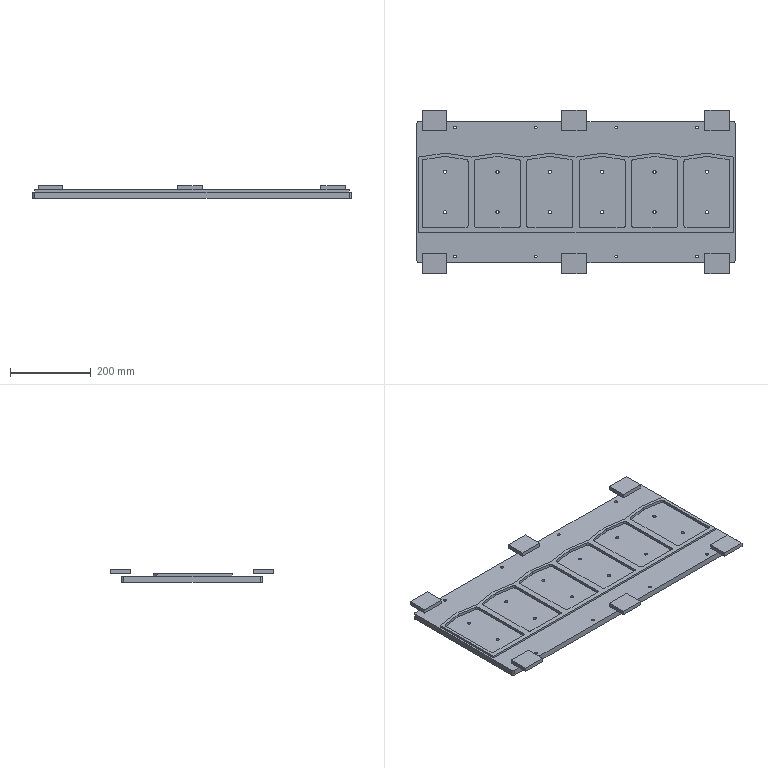Part | 7 solids | 168 faces | volume 4238061 mm3 | plane 94 | cylinder 74 | commonest cylinder face diameters 10 x34 8 x24 6.8 x16